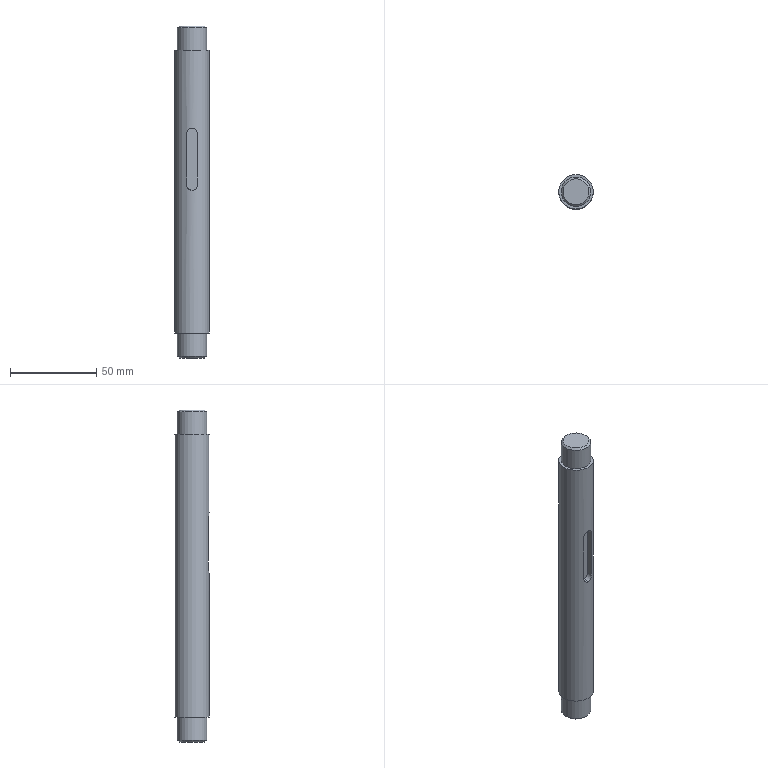Part | NX | features EXTRUDE 3, DATUM_CSYS 2, EXTRACT_DATUM_PLANE 2, SKETCH 2, CHAMFER 1, UNITE 1 | 1 solid | 16 faces | box 20 x 20 x 191.953 mm | volume 57075 mm3 | plane 7 | spline 4 | cylinder 3 | cone 2 | commonest cylinder face diameters 17 x2 20 x1
STEP:
#1=CARTESIAN_POINT('',(-10.,0.,81.75));
#2=VERTEX_POINT('',#1);
#3=CARTESIAN_POINT('',(0.,0.,81.75));
#4=DIRECTION('',(0.,0.,1.));
#5=DIRECTION('',(-1.,0.,0.));
#6=AXIS2_PLACEMENT_3D('',#3,#4,#5);
#7=CIRCLE('',#6,10.);
#8=EDGE_CURVE('',#2,#2,#7,.T.);
#9=ORIENTED_EDGE('',*,*,#8,.F.);
#10=EDGE_LOOP('',(#9));
#11=FACE_BOUND('',#10,.T.);
#12=CARTESIAN_POINT('',(10.,0.,-81.75));
#13=VERTEX_POINT('',#12);
#14=CARTESIAN_POINT('',(0.,0.,-81.75));
#15=DIRECTION('',(0.,0.,1.));
#16=DIRECTION('',(1.,0.,0.));
#17=AXIS2_PLACEMENT_3D('',#14,#15,#16);
#18=CIRCLE('',#17,10.);
#19=EDGE_CURVE('',#13,#13,#18,.T.);
#20=ORIENTED_EDGE('',*,*,#19,.T.);
#21=EDGE_LOOP('',(#20));
#22=FACE_BOUND('',#21,.T.);
#23=CARTESIAN_POINT('',(0.,-10.,0.75));
#24=VERTEX_POINT('',#23);
#25=CARTESIAN_POINT('',(-3.,-9.539,3.75));
#26=VERTEX_POINT('',#25);
#27=CARTESIAN_POINT('',(0.,-10.,0.75));
#28=CARTESIAN_POINT('',(-0.7973,-10.,0.75));
#29=CARTESIAN_POINT('',(-2.343,-9.775,1.405));
#30=CARTESIAN_POINT('',(-3.,-9.539,2.953));
#31=CARTESIAN_POINT('',(-3.,-9.539,3.75));
#32=B_SPLINE_CURVE_WITH_KNOTS('',3,(#27,#28,#29,#30,#31),.UNSPECIFIED.,.F.,.F.,(4,1,4),(0.,0.002356,0.004711),.UNSPECIFIED.);
#33=EDGE_CURVE('',#24,#26,#32,.T.);
#34=ORIENTED_EDGE('',*,*,#33,.T.);
#35=CARTESIAN_POINT('',(-3.,-9.539,33.75));
#36=VERTEX_POINT('',#35);
#37=CARTESIAN_POINT('',(-3.,-9.539,-81.75));
#38=DIRECTION('',(0.,0.,1.));
#39=VECTOR('',#38,1000.);
#40=LINE('',#37,#39);
#41=EDGE_CURVE('',#26,#36,#40,.T.);
#42=ORIENTED_EDGE('',*,*,#41,.T.);
#43=CARTESIAN_POINT('',(0.,-10.,36.75));
#44=VERTEX_POINT('',#43);
#45=CARTESIAN_POINT('',(-3.,-9.539,33.75));
#46=CARTESIAN_POINT('',(-3.,-9.539,34.547));
#47=CARTESIAN_POINT('',(-2.345,-9.775,36.093));
#48=CARTESIAN_POINT('',(-0.797,-10.,36.75));
#49=CARTESIAN_POINT('',(0.,-10.,36.75));
#50=B_SPLINE_CURVE_WITH_KNOTS('',3,(#45,#46,#47,#48,#49),.UNSPECIFIED.,.F.,.F.,(4,1,4),(0.,0.002356,0.004711),.UNSPECIFIED.);
#51=EDGE_CURVE('',#36,#44,#50,.T.);
#52=ORIENTED_EDGE('',*,*,#51,.T.);
#53=CARTESIAN_POINT('',(3.,-9.539,33.75));
#54=VERTEX_POINT('',#53);
#55=CARTESIAN_POINT('',(0.,-10.,36.75));
#56=CARTESIAN_POINT('',(0.7973,-10.,36.75));
#57=CARTESIAN_POINT('',(2.343,-9.775,36.095));
#58=CARTESIAN_POINT('',(3.,-9.539,34.547));
#59=CARTESIAN_POINT('',(3.,-9.539,33.75));
#60=B_SPLINE_CURVE_WITH_KNOTS('',3,(#55,#56,#57,#58,#59),.UNSPECIFIED.,.F.,.F.,(4,1,4),(0.,0.002356,0.004711),.UNSPECIFIED.);
#61=EDGE_CURVE('',#44,#54,#60,.T.);
#62=ORIENTED_EDGE('',*,*,#61,.T.);
#63=CARTESIAN_POINT('',(3.,-9.539,3.75));
#64=VERTEX_POINT('',#63);
#65=CARTESIAN_POINT('',(3.,-9.539,-81.75));
#66=DIRECTION('',(0.,0.,1.));
#67=VECTOR('',#66,1000.);
#68=LINE('',#65,#67);
#69=EDGE_CURVE('',#54,#64,#68,.F.);
#70=ORIENTED_EDGE('',*,*,#69,.T.);
#71=CARTESIAN_POINT('',(3.,-9.539,3.75));
#72=CARTESIAN_POINT('',(3.,-9.539,2.953));
#73=CARTESIAN_POINT('',(2.345,-9.775,1.407));
#74=CARTESIAN_POINT('',(0.797,-10.,0.75));
#75=CARTESIAN_POINT('',(0.,-10.,0.75));
#76=B_SPLINE_CURVE_WITH_KNOTS('',3,(#71,#72,#73,#74,#75),.UNSPECIFIED.,.F.,.F.,(4,1,4),(0.,0.002356,0.004711),.UNSPECIFIED.);
#77=EDGE_CURVE('',#64,#24,#76,.T.);
#78=ORIENTED_EDGE('',*,*,#77,.T.);
#79=EDGE_LOOP('',(#34,#42,#52,#62,#70,#78));
#80=FACE_BOUND('',#79,.T.);
#81=CARTESIAN_POINT('',(0.,0.,-81.75));
#82=DIRECTION('',(0.,0.,1.));
#83=DIRECTION('',(1.,0.,0.));
#84=AXIS2_PLACEMENT_3D('',#81,#82,#83);
#85=CYLINDRICAL_SURFACE('',#84,10.);
#86=ADVANCED_FACE('',(#11,#22,#80),#85,.T.);
#87=CARTESIAN_POINT('',(8.5,0.,-81.75));
#88=VERTEX_POINT('',#87);
#89=CARTESIAN_POINT('',(0.,0.,-81.75));
#90=DIRECTION('',(0.,0.,1.));
#91=DIRECTION('',(1.,0.,0.));
#92=AXIS2_PLACEMENT_3D('',#89,#90,#91);
#93=CIRCLE('',#92,8.5);
#94=EDGE_CURVE('',#88,#88,#93,.F.);
#95=ORIENTED_EDGE('',*,*,#94,.F.);
#96=EDGE_LOOP('',(#95));
#97=FACE_BOUND('',#96,.T.);
#98=ORIENTED_EDGE('',*,*,#19,.F.);
#99=EDGE_LOOP('',(#98));
#100=FACE_BOUND('',#99,.T.);
#101=CARTESIAN_POINT('',(0.,0.,-81.75));
#102=DIRECTION('',(0.,0.,1.));
#103=DIRECTION('',(1.,0.,0.));
#104=AXIS2_PLACEMENT_3D('',#101,#102,#103);
#105=PLANE('',#104);
#106=ADVANCED_FACE('',(#97,#100),#105,.F.);
#107=CARTESIAN_POINT('',(8.5,0.,81.75));
#108=VERTEX_POINT('',#107);
#109=CARTESIAN_POINT('',(0.,0.,81.75));
#110=DIRECTION('',(0.,0.,1.));
#111=DIRECTION('',(1.,0.,0.));
#112=AXIS2_PLACEMENT_3D('',#109,#110,#111);
#113=CIRCLE('',#112,8.5);
#114=EDGE_CURVE('',#108,#108,#113,.F.);
#115=ORIENTED_EDGE('',*,*,#114,.T.);
#116=EDGE_LOOP('',(#115));
#117=FACE_BOUND('',#116,.T.);
#118=ORIENTED_EDGE('',*,*,#8,.T.);
#119=EDGE_LOOP('',(#118));
#120=FACE_BOUND('',#119,.T.);
#121=CARTESIAN_POINT('',(0.,0.,81.75));
#122=DIRECTION('',(0.,0.,1.));
#123=DIRECTION('',(1.,0.,0.));
#124=AXIS2_PLACEMENT_3D('',#121,#122,#123);
#125=PLANE('',#124);
#126=ADVANCED_FACE('',(#117,#120),#125,.T.);
#127=CARTESIAN_POINT('',(-7.5,0.,95.75));
#128=VERTEX_POINT('',#127);
#129=CARTESIAN_POINT('',(0.,0.,95.75));
#130=DIRECTION('',(0.,0.,-1.));
#131=DIRECTION('',(-1.,0.,0.));
#132=AXIS2_PLACEMENT_3D('',#129,#130,#131);
#133=CIRCLE('',#132,7.5);
#134=EDGE_CURVE('',#128,#128,#133,.F.);
#135=ORIENTED_EDGE('',*,*,#134,.T.);
#136=EDGE_LOOP('',(#135));
#137=FACE_BOUND('',#136,.T.);
#138=CARTESIAN_POINT('',(0.,0.,95.75));
#139=DIRECTION('',(0.,0.,-1.));
#140=DIRECTION('',(-1.,0.,0.));
#141=AXIS2_PLACEMENT_3D('',#138,#139,#140);
#142=PLANE('',#141);
#143=ADVANCED_FACE('',(#137),#142,.F.);
#144=CARTESIAN_POINT('',(-8.5,0.,94.75));
#145=VERTEX_POINT('',#144);
#146=CARTESIAN_POINT('',(0.,0.,94.75));
#147=DIRECTION('',(0.,0.,-1.));
#148=DIRECTION('',(-1.,0.,0.));
#149=AXIS2_PLACEMENT_3D('',#146,#147,#148);
#150=CIRCLE('',#149,8.5);
#151=EDGE_CURVE('',#145,#145,#150,.T.);
#152=ORIENTED_EDGE('',*,*,#151,.T.);
#153=EDGE_LOOP('',(#152));
#154=FACE_BOUND('',#153,.T.);
#155=ORIENTED_EDGE('',*,*,#114,.F.);
#156=EDGE_LOOP('',(#155));
#157=FACE_BOUND('',#156,.T.);
#158=CARTESIAN_POINT('',(0.,0.,-96.203));
#159=DIRECTION('',(0.,0.,1.));
#160=DIRECTION('',(1.,0.,0.));
#161=AXIS2_PLACEMENT_3D('',#158,#159,#160);
#162=CYLINDRICAL_SURFACE('',#161,8.5);
#163=ADVANCED_FACE('',(#154,#157),#162,.T.);
#164=CARTESIAN_POINT('',(-8.5,0.,-95.203));
#165=VERTEX_POINT('',#164);
#166=CARTESIAN_POINT('',(0.,0.,-95.203));
#167=DIRECTION('',(0.,0.,-1.));
#168=DIRECTION('',(-1.,0.,0.));
#169=AXIS2_PLACEMENT_3D('',#166,#167,#168);
#170=CIRCLE('',#169,8.5);
#171=EDGE_CURVE('',#165,#165,#170,.F.);
#172=ORIENTED_EDGE('',*,*,#171,.T.);
#173=EDGE_LOOP('',(#172));
#174=FACE_BOUND('',#173,.T.);
#175=ORIENTED_EDGE('',*,*,#94,.T.);
#176=EDGE_LOOP('',(#175));
#177=FACE_BOUND('',#176,.T.);
#178=CARTESIAN_POINT('',(0.,0.,-96.203));
#179=DIRECTION('',(0.,0.,1.));
#180=DIRECTION('',(1.,0.,0.));
#181=AXIS2_PLACEMENT_3D('',#178,#179,#180);
#182=CYLINDRICAL_SURFACE('',#181,8.5);
#183=ADVANCED_FACE('',(#174,#177),#182,.T.);
#184=CARTESIAN_POINT('',(-7.5,0.,-96.203));
#185=VERTEX_POINT('',#184);
#186=CARTESIAN_POINT('',(0.,0.,-96.203));
#187=DIRECTION('',(0.,0.,-1.));
#188=DIRECTION('',(-1.,0.,0.));
#189=AXIS2_PLACEMENT_3D('',#186,#187,#188);
#190=CIRCLE('',#189,7.5);
#191=EDGE_CURVE('',#185,#185,#190,.T.);
#192=ORIENTED_EDGE('',*,*,#191,.T.);
#193=EDGE_LOOP('',(#192));
#194=FACE_BOUND('',#193,.T.);
#195=CARTESIAN_POINT('',(0.,0.,-96.203));
#196=DIRECTION('',(0.,0.,-1.));
#197=DIRECTION('',(-1.,0.,0.));
#198=AXIS2_PLACEMENT_3D('',#195,#196,#197);
#199=PLANE('',#198);
#200=ADVANCED_FACE('',(#194),#199,.T.);
#201=CARTESIAN_POINT('',(-3.,-6.5,3.75));
#202=VERTEX_POINT('',#201);
#203=CARTESIAN_POINT('',(-3.,-161.793,3.75));
#204=DIRECTION('',(0.,1.,0.));
#205=VECTOR('',#204,1000.);
#206=LINE('',#203,#205);
#207=EDGE_CURVE('',#202,#26,#206,.F.);
#208=ORIENTED_EDGE('',*,*,#207,.F.);
#209=CARTESIAN_POINT('',(-3.,-6.5,33.75));
#210=VERTEX_POINT('',#209);
#211=CARTESIAN_POINT('',(-3.,-6.5,33.75));
#212=DIRECTION('',(0.,0.,-1.));
#213=VECTOR('',#212,1000.);
#214=LINE('',#211,#213);
#215=EDGE_CURVE('',#202,#210,#214,.F.);
#216=ORIENTED_EDGE('',*,*,#215,.T.);
#217=CARTESIAN_POINT('',(-3.,-161.793,33.75));
#218=DIRECTION('',(0.,1.,0.));
#219=VECTOR('',#218,1000.);
#220=LINE('',#217,#219);
#221=EDGE_CURVE('',#210,#36,#220,.F.);
#222=ORIENTED_EDGE('',*,*,#221,.T.);
#223=ORIENTED_EDGE('',*,*,#41,.F.);
#224=EDGE_LOOP('',(#208,#216,#222,#223));
#225=FACE_BOUND('',#224,.T.);
#226=CARTESIAN_POINT('',(-3.,-161.793,33.75));
#227=DIRECTION('',(1.,0.,0.));
#228=DIRECTION('',(0.,0.,-1.));
#229=AXIS2_PLACEMENT_3D('',#226,#227,#228);
#230=PLANE('',#229);
#231=ADVANCED_FACE('',(#225),#230,.T.);
#232=CARTESIAN_POINT('',(0.,-6.5,0.75));
#233=VERTEX_POINT('',#232);
#234=CARTESIAN_POINT('',(0.,-161.793,0.75));
#235=DIRECTION('',(0.,1.,0.));
#236=VECTOR('',#235,1000.);
#237=LINE('',#234,#236);
#238=EDGE_CURVE('',#233,#24,#237,.F.);
#239=ORIENTED_EDGE('',*,*,#238,.F.);
#240=CARTESIAN_POINT('',(-3.,-6.5,3.75));
#241=CARTESIAN_POINT('',(-3.,-6.5,2.953));
#242=CARTESIAN_POINT('',(-2.671,-6.5,2.178));
#243=CARTESIAN_POINT('',(-1.571,-6.5,1.079));
#244=CARTESIAN_POINT('',(-0.7973,-6.5,0.75));
#245=CARTESIAN_POINT('',(0.,-6.5,0.75));
#246=B_SPLINE_CURVE_WITH_KNOTS('',3,(#240,#241,#242,#243,#244,#245),.UNSPECIFIED.,.F.,.F.,(4,2,4),(0.,0.5,1.),.UNSPECIFIED.);
#247=EDGE_CURVE('',#233,#202,#246,.F.);
#248=ORIENTED_EDGE('',*,*,#247,.T.);
#249=ORIENTED_EDGE('',*,*,#207,.T.);
#250=ORIENTED_EDGE('',*,*,#33,.F.);
#251=EDGE_LOOP('',(#239,#248,#249,#250));
#252=FACE_BOUND('',#251,.T.);
#253=CARTESIAN_POINT('',(-3.,-10.021,3.75));
#254=CARTESIAN_POINT('',(-3.,-6.5,3.75));
#255=CARTESIAN_POINT('',(-3.,-10.021,2.953));
#256=CARTESIAN_POINT('',(-3.,-6.5,2.953));
#257=CARTESIAN_POINT('',(-2.343,-10.021,1.405));
#258=CARTESIAN_POINT('',(-2.343,-6.5,1.405));
#259=CARTESIAN_POINT('',(-0.7973,-10.021,0.75));
#260=CARTESIAN_POINT('',(-0.7973,-6.5,0.75));
#261=CARTESIAN_POINT('',(0.,-10.021,0.75));
#262=CARTESIAN_POINT('',(0.,-6.5,0.75));
#263=B_SPLINE_SURFACE_WITH_KNOTS('',3,1,((#253,#254),(#255,#256),(#257,#258),(#259,#260),(#261,#262)),.SURF_OF_LINEAR_EXTRUSION.,.F.,.F.,.F.,(4,1,4),(2,2),(0.,0.5,1.),(0.,1.),.UNSPECIFIED.);
#264=ADVANCED_FACE('',(#252),#263,.T.);
#265=CARTESIAN_POINT('',(3.,-6.5,3.75));
#266=VERTEX_POINT('',#265);
#267=CARTESIAN_POINT('',(3.,-161.793,3.75));
#268=DIRECTION('',(0.,1.,0.));
#269=VECTOR('',#268,1000.);
#270=LINE('',#267,#269);
#271=EDGE_CURVE('',#266,#64,#270,.F.);
#272=ORIENTED_EDGE('',*,*,#271,.F.);
#273=CARTESIAN_POINT('',(0.,-6.5,0.75));
#274=CARTESIAN_POINT('',(0.7973,-6.5,0.75));
#275=CARTESIAN_POINT('',(1.572,-6.5,1.079));
#276=CARTESIAN_POINT('',(2.671,-6.5,2.179));
#277=CARTESIAN_POINT('',(3.,-6.5,2.953));
#278=CARTESIAN_POINT('',(3.,-6.5,3.75));
#279=B_SPLINE_CURVE_WITH_KNOTS('',3,(#273,#274,#275,#276,#277,#278),.UNSPECIFIED.,.F.,.F.,(4,2,4),(0.,0.5,1.),.UNSPECIFIED.);
#280=EDGE_CURVE('',#266,#233,#279,.F.);
#281=ORIENTED_EDGE('',*,*,#280,.T.);
#282=ORIENTED_EDGE('',*,*,#238,.T.);
#283=ORIENTED_EDGE('',*,*,#77,.F.);
#284=EDGE_LOOP('',(#272,#281,#282,#283));
#285=FACE_BOUND('',#284,.T.);
#286=CARTESIAN_POINT('',(0.,-10.021,0.75));
#287=CARTESIAN_POINT('',(0.,-6.5,0.75));
#288=CARTESIAN_POINT('',(0.7973,-10.021,0.75));
#289=CARTESIAN_POINT('',(0.7973,-6.5,0.75));
#290=CARTESIAN_POINT('',(2.345,-10.021,1.407));
#291=CARTESIAN_POINT('',(2.345,-6.5,1.407));
#292=CARTESIAN_POINT('',(3.,-10.021,2.953));
#293=CARTESIAN_POINT('',(3.,-6.5,2.953));
#294=CARTESIAN_POINT('',(3.,-10.021,3.75));
#295=CARTESIAN_POINT('',(3.,-6.5,3.75));
#296=B_SPLINE_SURFACE_WITH_KNOTS('',3,1,((#286,#287),(#288,#289),(#290,#291),(#292,#293),(#294,#295)),.SURF_OF_LINEAR_EXTRUSION.,.F.,.F.,.F.,(4,1,4),(2,2),(0.,0.5,1.),(0.,1.),.UNSPECIFIED.);
#297=ADVANCED_FACE('',(#285),#296,.T.);
#298=CARTESIAN_POINT('',(3.,-6.5,33.75));
#299=VERTEX_POINT('',#298);
#300=CARTESIAN_POINT('',(3.,-161.793,33.75));
#301=DIRECTION('',(0.,1.,0.));
#302=VECTOR('',#301,1000.);
#303=LINE('',#300,#302);
#304=EDGE_CURVE('',#299,#54,#303,.F.);
#305=ORIENTED_EDGE('',*,*,#304,.F.);
#306=CARTESIAN_POINT('',(3.,-6.5,3.75));
#307=DIRECTION('',(0.,0.,1.));
#308=VECTOR('',#307,1000.);
#309=LINE('',#306,#308);
#310=EDGE_CURVE('',#299,#266,#309,.F.);
#311=ORIENTED_EDGE('',*,*,#310,.T.);
#312=ORIENTED_EDGE('',*,*,#271,.T.);
#313=ORIENTED_EDGE('',*,*,#69,.F.);
#314=EDGE_LOOP('',(#305,#311,#312,#313));
#315=FACE_BOUND('',#314,.T.);
#316=CARTESIAN_POINT('',(3.,-161.793,3.75));
#317=DIRECTION('',(-1.,0.,0.));
#318=DIRECTION('',(0.,0.,1.));
#319=AXIS2_PLACEMENT_3D('',#316,#317,#318);
#320=PLANE('',#319);
#321=ADVANCED_FACE('',(#315),#320,.T.);
#322=CARTESIAN_POINT('',(0.,-6.5,36.75));
#323=VERTEX_POINT('',#322);
#324=CARTESIAN_POINT('',(0.,-161.793,36.75));
#325=DIRECTION('',(0.,1.,0.));
#326=VECTOR('',#325,1000.);
#327=LINE('',#324,#326);
#328=EDGE_CURVE('',#323,#44,#327,.F.);
#329=ORIENTED_EDGE('',*,*,#328,.F.);
#330=CARTESIAN_POINT('',(3.,-6.5,33.75));
#331=CARTESIAN_POINT('',(3.,-6.5,34.547));
#332=CARTESIAN_POINT('',(2.671,-6.5,35.322));
#333=CARTESIAN_POINT('',(1.571,-6.5,36.421));
#334=CARTESIAN_POINT('',(0.7973,-6.5,36.75));
#335=CARTESIAN_POINT('',(0.,-6.5,36.75));
#336=B_SPLINE_CURVE_WITH_KNOTS('',3,(#330,#331,#332,#333,#334,#335),.UNSPECIFIED.,.F.,.F.,(4,2,4),(0.,0.5,1.),.UNSPECIFIED.);
#337=EDGE_CURVE('',#323,#299,#336,.F.);
#338=ORIENTED_EDGE('',*,*,#337,.T.);
#339=ORIENTED_EDGE('',*,*,#304,.T.);
#340=ORIENTED_EDGE('',*,*,#61,.F.);
#341=EDGE_LOOP('',(#329,#338,#339,#340));
#342=FACE_BOUND('',#341,.T.);
#343=CARTESIAN_POINT('',(3.,-10.021,33.75));
#344=CARTESIAN_POINT('',(3.,-6.5,33.75));
#345=CARTESIAN_POINT('',(3.,-10.021,34.547));
#346=CARTESIAN_POINT('',(3.,-6.5,34.547));
#347=CARTESIAN_POINT('',(2.343,-10.021,36.095));
#348=CARTESIAN_POINT('',(2.343,-6.5,36.095));
#349=CARTESIAN_POINT('',(0.7973,-10.021,36.75));
#350=CARTESIAN_POINT('',(0.7973,-6.5,36.75));
#351=CARTESIAN_POINT('',(0.,-10.021,36.75));
#352=CARTESIAN_POINT('',(0.,-6.5,36.75));
#353=B_SPLINE_SURFACE_WITH_KNOTS('',3,1,((#343,#344),(#345,#346),(#347,#348),(#349,#350),(#351,#352)),.SURF_OF_LINEAR_EXTRUSION.,.F.,.F.,.F.,(4,1,4),(2,2),(0.,0.5,1.),(0.,1.),.UNSPECIFIED.);
#354=ADVANCED_FACE('',(#342),#353,.T.);
#355=ORIENTED_EDGE('',*,*,#221,.F.);
#356=CARTESIAN_POINT('',(0.,-6.5,36.75));
#357=CARTESIAN_POINT('',(-0.7973,-6.5,36.75));
#358=CARTESIAN_POINT('',(-1.572,-6.5,36.421));
#359=CARTESIAN_POINT('',(-2.671,-6.5,35.321));
#360=CARTESIAN_POINT('',(-3.,-6.5,34.547));
#361=CARTESIAN_POINT('',(-3.,-6.5,33.75));
#362=B_SPLINE_CURVE_WITH_KNOTS('',3,(#356,#357,#358,#359,#360,#361),.UNSPECIFIED.,.F.,.F.,(4,2,4),(0.,0.5,1.),.UNSPECIFIED.);
#363=EDGE_CURVE('',#210,#323,#362,.F.);
#364=ORIENTED_EDGE('',*,*,#363,.T.);
#365=ORIENTED_EDGE('',*,*,#328,.T.);
#366=ORIENTED_EDGE('',*,*,#51,.F.);
#367=EDGE_LOOP('',(#355,#364,#365,#366));
#368=FACE_BOUND('',#367,.T.);
#369=CARTESIAN_POINT('',(0.,-10.021,36.75));
#370=CARTESIAN_POINT('',(0.,-6.5,36.75));
#371=CARTESIAN_POINT('',(-0.7973,-10.021,36.75));
#372=CARTESIAN_POINT('',(-0.7973,-6.5,36.75));
#373=CARTESIAN_POINT('',(-2.345,-10.021,36.093));
#374=CARTESIAN_POINT('',(-2.345,-6.5,36.093));
#375=CARTESIAN_POINT('',(-3.,-10.021,34.547));
#376=CARTESIAN_POINT('',(-3.,-6.5,34.547));
#377=CARTESIAN_POINT('',(-3.,-10.021,33.75));
#378=CARTESIAN_POINT('',(-3.,-6.5,33.75));
#379=B_SPLINE_SURFACE_WITH_KNOTS('',3,1,((#369,#370),(#371,#372),(#373,#374),(#375,#376),(#377,#378)),.SURF_OF_LINEAR_EXTRUSION.,.F.,.F.,.F.,(4,1,4),(2,2),(0.,0.5,1.),(0.,1.),.UNSPECIFIED.);
#380=ADVANCED_FACE('',(#368),#379,.T.);
#381=ORIENTED_EDGE('',*,*,#215,.F.);
#382=ORIENTED_EDGE('',*,*,#247,.F.);
#383=ORIENTED_EDGE('',*,*,#280,.F.);
#384=ORIENTED_EDGE('',*,*,#310,.F.);
#385=ORIENTED_EDGE('',*,*,#337,.F.);
#386=ORIENTED_EDGE('',*,*,#363,.F.);
#387=EDGE_LOOP('',(#381,#382,#383,#384,#385,#386));
#388=FACE_BOUND('',#387,.T.);
#389=CARTESIAN_POINT('',(-2.121,-6.5,1.628));
#390=DIRECTION('',(0.,1.,0.));
#391=DIRECTION('',(0.,0.,1.));
#392=AXIS2_PLACEMENT_3D('',#389,#390,#391);
#393=PLANE('',#392);
#394=ADVANCED_FACE('',(#388),#393,.F.);
#395=ORIENTED_EDGE('',*,*,#134,.F.);
#396=EDGE_LOOP('',(#395));
#397=FACE_BOUND('',#396,.T.);
#398=ORIENTED_EDGE('',*,*,#151,.F.);
#399=EDGE_LOOP('',(#398));
#400=FACE_BOUND('',#399,.T.);
#401=CARTESIAN_POINT('',(0.,0.,94.75));
#402=DIRECTION('',(0.,0.,-1.));
#403=DIRECTION('',(-1.,0.,0.));
#404=AXIS2_PLACEMENT_3D('',#401,#402,#403);
#405=CONICAL_SURFACE('',#404,8.5,0.7854);
#406=ADVANCED_FACE('',(#397,#400),#405,.T.);
#407=ORIENTED_EDGE('',*,*,#171,.F.);
#408=EDGE_LOOP('',(#407));
#409=FACE_BOUND('',#408,.T.);
#410=ORIENTED_EDGE('',*,*,#191,.F.);
#411=EDGE_LOOP('',(#410));
#412=FACE_BOUND('',#411,.T.);
#413=CARTESIAN_POINT('',(0.,0.,-96.203));
#414=DIRECTION('',(0.,0.,1.));
#415=DIRECTION('',(1.,0.,0.));
#416=AXIS2_PLACEMENT_3D('',#413,#414,#415);
#417=CONICAL_SURFACE('',#416,7.5,0.7854);
#418=ADVANCED_FACE('',(#409,#412),#417,.T.);
#419=CLOSED_SHELL('',(#86,#106,#126,#143,#163,#183,#200,#231,#264,#297,#321,#354,#380,#394,#406,#418));
#420=MANIFOLD_SOLID_BREP('',#419);
#421=(LENGTH_UNIT()NAMED_UNIT(*)SI_UNIT(.MILLI.,.METRE.));
#422=UNCERTAINTY_MEASURE_WITH_UNIT(LENGTH_MEASURE(0.0508),#421,'','');
#423=(NAMED_UNIT(*)PLANE_ANGLE_UNIT()SI_UNIT($,.RADIAN.));
#424=(NAMED_UNIT(*)SI_UNIT($,.STERADIAN.)SOLID_ANGLE_UNIT());
#425=(GEOMETRIC_REPRESENTATION_CONTEXT(3)GLOBAL_UNCERTAINTY_ASSIGNED_CONTEXT((#422))GLOBAL_UNIT_ASSIGNED_CONTEXT((#421,#423,#424))REPRESENTATION_CONTEXT('',''));
#426=ADVANCED_BREP_SHAPE_REPRESENTATION('',(#420),#425);